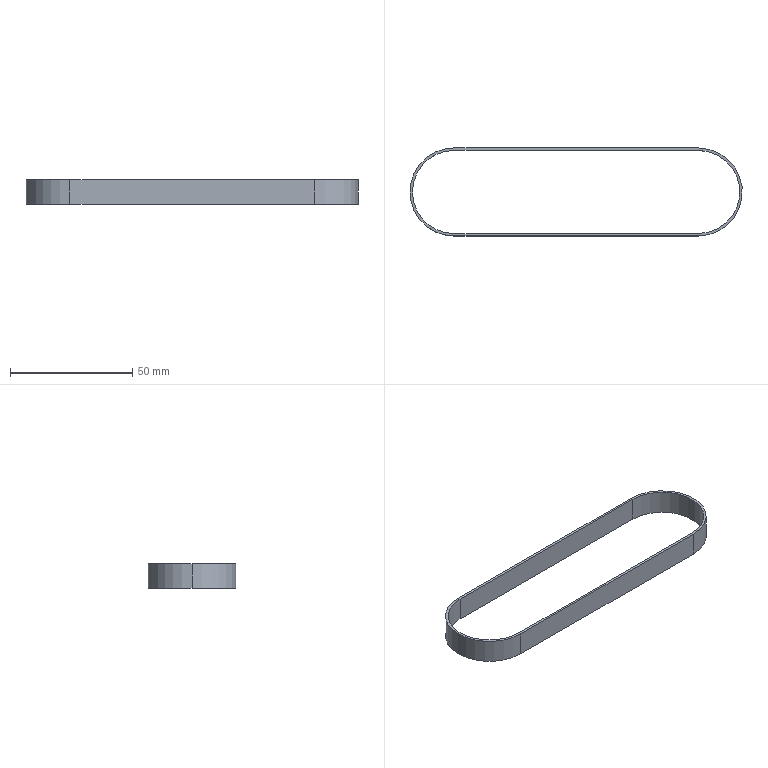Part | STEP file | Belt V1.201001 | 1 solid | 12 faces | box 136 x 36 x 10 mm | volume 3100 mm3 | cylinder 6 | plane 6 | commonest cylinder face diameters 34 x3 36 x3
STEP:
#1=CARTESIAN_POINT('',(0.,0.,0.));
#2=DIRECTION('',(0.,0.,1.));
#3=DIRECTION('',(1.,0.,0.));
#4=AXIS2_PLACEMENT_3D('',#1,#2,#3);
#5=CARTESIAN_POINT('',(-50.,17.,5.));
#6=VERTEX_POINT('',#5);
#7=CARTESIAN_POINT('',(-50.,17.,-5.));
#8=VERTEX_POINT('',#7);
#9=CARTESIAN_POINT('',(-50.,17.,5.));
#10=DIRECTION('',(0.,0.,-1.));
#11=VECTOR('',#10,1.);
#12=LINE('',#9,#11);
#13=CARTESIAN_POINT('',(-50.,0.,5.));
#14=DIRECTION('',(0.,0.,-1.));
#15=DIRECTION('',(-1.,0.,0.));
#16=AXIS2_PLACEMENT_3D('',#13,#14,#15);
#17=CYLINDRICAL_SURFACE('',#16,17.);
#18=CARTESIAN_POINT('',(1.571,0.));
#19=DIRECTION('',(0.,1.));
#20=VECTOR('',#19,1.);
#21=LINE('',#18,#20);
#22=(GEOMETRIC_REPRESENTATION_CONTEXT(2)PARAMETRIC_REPRESENTATION_CONTEXT()REPRESENTATION_CONTEXT('',''));
#23=DEFINITIONAL_REPRESENTATION('',(#21),#22);
#24=PCURVE('',#17,#23);
#25=CARTESIAN_POINT('',(-50.,17.,5.));
#26=DIRECTION('',(0.,-1.,0.));
#27=DIRECTION('',(0.,0.,-1.));
#28=AXIS2_PLACEMENT_3D('',#25,#26,#27);
#29=PLANE('',#28);
#30=CARTESIAN_POINT('',(0.,0.));
#31=DIRECTION('',(1.,0.));
#32=VECTOR('',#31,1.);
#33=LINE('',#30,#32);
#34=(GEOMETRIC_REPRESENTATION_CONTEXT(2)PARAMETRIC_REPRESENTATION_CONTEXT()REPRESENTATION_CONTEXT('',''));
#35=DEFINITIONAL_REPRESENTATION('',(#33),#34);
#36=PCURVE('',#29,#35);
#37=SURFACE_CURVE('',#12,(#24,#36),.PCURVE_S1.);
#38=EDGE_CURVE('',#6,#8,#37,.T.);
#39=ORIENTED_EDGE('',*,*,#38,.T.);
#40=CARTESIAN_POINT('',(-67.,0.,-5.));
#41=VERTEX_POINT('',#40);
#42=CARTESIAN_POINT('',(-50.,0.,-5.));
#43=DIRECTION('',(0.,0.,1.));
#44=DIRECTION('',(1.,0.,0.));
#45=AXIS2_PLACEMENT_3D('',#42,#43,#44);
#46=CIRCLE('',#45,17.);
#47=CARTESIAN_POINT('',(3.142,10.));
#48=DIRECTION('',(-1.,0.));
#49=VECTOR('',#48,1.);
#50=LINE('',#47,#49);
#51=(GEOMETRIC_REPRESENTATION_CONTEXT(2)PARAMETRIC_REPRESENTATION_CONTEXT()REPRESENTATION_CONTEXT('',''));
#52=DEFINITIONAL_REPRESENTATION('',(#50),#51);
#53=PCURVE('',#17,#52);
#54=CARTESIAN_POINT('',(-50.,0.,-5.));
#55=DIRECTION('',(0.,0.,1.));
#56=DIRECTION('',(1.,0.,0.));
#57=AXIS2_PLACEMENT_3D('',#54,#55,#56);
#58=PLANE('',#57);
#59=CARTESIAN_POINT('',(0.,0.));
#60=DIRECTION('',(1.,0.));
#61=AXIS2_PLACEMENT_2D('',#59,#60);
#62=CIRCLE('',#61,17.);
#63=(GEOMETRIC_REPRESENTATION_CONTEXT(2)PARAMETRIC_REPRESENTATION_CONTEXT()REPRESENTATION_CONTEXT('',''));
#64=DEFINITIONAL_REPRESENTATION('',(#62),#63);
#65=PCURVE('',#58,#64);
#66=SURFACE_CURVE('',#46,(#53,#65),.PCURVE_S1.);
#67=EDGE_CURVE('',#8,#41,#66,.T.);
#68=ORIENTED_EDGE('',*,*,#67,.T.);
#69=CARTESIAN_POINT('',(-67.,0.,5.));
#70=VERTEX_POINT('',#69);
#71=CARTESIAN_POINT('',(-67.,0.,5.));
#72=DIRECTION('',(0.,0.,-1.));
#73=VECTOR('',#72,1.);
#74=LINE('',#71,#73);
#75=CARTESIAN_POINT('',(0.,0.));
#76=DIRECTION('',(0.,1.));
#77=VECTOR('',#76,1.);
#78=LINE('',#75,#77);
#79=(GEOMETRIC_REPRESENTATION_CONTEXT(2)PARAMETRIC_REPRESENTATION_CONTEXT()REPRESENTATION_CONTEXT('',''));
#80=DEFINITIONAL_REPRESENTATION('',(#78),#79);
#81=PCURVE('',#17,#80);
#82=CARTESIAN_POINT('',(-50.,0.,5.));
#83=DIRECTION('',(0.,0.,-1.));
#84=DIRECTION('',(-1.,0.,0.));
#85=AXIS2_PLACEMENT_3D('',#82,#83,#84);
#86=CYLINDRICAL_SURFACE('',#85,17.);
#87=CARTESIAN_POINT('',(6.283,0.));
#88=DIRECTION('',(0.,1.));
#89=VECTOR('',#88,1.);
#90=LINE('',#87,#89);
#91=(GEOMETRIC_REPRESENTATION_CONTEXT(2)PARAMETRIC_REPRESENTATION_CONTEXT()REPRESENTATION_CONTEXT('',''));
#92=DEFINITIONAL_REPRESENTATION('',(#90),#91);
#93=PCURVE('',#86,#92);
#94=SURFACE_CURVE('',#74,(#81,#93),.PCURVE_S1.);
#95=EDGE_CURVE('',#70,#41,#94,.T.);
#96=ORIENTED_EDGE('',*,*,#95,.F.);
#97=CARTESIAN_POINT('',(-50.,0.,5.));
#98=DIRECTION('',(0.,0.,1.));
#99=DIRECTION('',(1.,0.,0.));
#100=AXIS2_PLACEMENT_3D('',#97,#98,#99);
#101=CIRCLE('',#100,17.);
#102=CARTESIAN_POINT('',(3.142,0.));
#103=DIRECTION('',(-1.,0.));
#104=VECTOR('',#103,1.);
#105=LINE('',#102,#104);
#106=(GEOMETRIC_REPRESENTATION_CONTEXT(2)PARAMETRIC_REPRESENTATION_CONTEXT()REPRESENTATION_CONTEXT('',''));
#107=DEFINITIONAL_REPRESENTATION('',(#105),#106);
#108=PCURVE('',#17,#107);
#109=CARTESIAN_POINT('',(-50.,0.,5.));
#110=DIRECTION('',(0.,0.,1.));
#111=DIRECTION('',(1.,0.,0.));
#112=AXIS2_PLACEMENT_3D('',#109,#110,#111);
#113=PLANE('',#112);
#114=CARTESIAN_POINT('',(0.,0.));
#115=DIRECTION('',(1.,0.));
#116=AXIS2_PLACEMENT_2D('',#114,#115);
#117=CIRCLE('',#116,17.);
#118=(GEOMETRIC_REPRESENTATION_CONTEXT(2)PARAMETRIC_REPRESENTATION_CONTEXT()REPRESENTATION_CONTEXT('',''));
#119=DEFINITIONAL_REPRESENTATION('',(#117),#118);
#120=PCURVE('',#113,#119);
#121=SURFACE_CURVE('',#101,(#108,#120),.PCURVE_S1.);
#122=EDGE_CURVE('',#6,#70,#121,.T.);
#123=ORIENTED_EDGE('',*,*,#122,.F.);
#124=EDGE_LOOP('',(#39,#68,#96,#123));
#125=FACE_BOUND('',#124,.F.);
#126=ADVANCED_FACE('',(#125),#17,.F.);
#127=CARTESIAN_POINT('',(-68.,0.,5.));
#128=VERTEX_POINT('',#127);
#129=CARTESIAN_POINT('',(-50.,-18.,5.));
#130=VERTEX_POINT('',#129);
#131=CARTESIAN_POINT('',(-50.,0.,5.));
#132=DIRECTION('',(0.,0.,1.));
#133=DIRECTION('',(1.,0.,0.));
#134=AXIS2_PLACEMENT_3D('',#131,#132,#133);
#135=CIRCLE('',#134,18.);
#136=CARTESIAN_POINT('',(-50.,0.,5.));
#137=DIRECTION('',(0.,0.,-1.));
#138=DIRECTION('',(-1.,0.,0.));
#139=AXIS2_PLACEMENT_3D('',#136,#137,#138);
#140=CYLINDRICAL_SURFACE('',#139,18.);
#141=CARTESIAN_POINT('',(9.425,0.));
#142=DIRECTION('',(-1.,0.));
#143=VECTOR('',#142,1.);
#144=LINE('',#141,#143);
#145=(GEOMETRIC_REPRESENTATION_CONTEXT(2)PARAMETRIC_REPRESENTATION_CONTEXT()REPRESENTATION_CONTEXT('',''));
#146=DEFINITIONAL_REPRESENTATION('',(#144),#145);
#147=PCURVE('',#140,#146);
#148=CARTESIAN_POINT('',(0.,0.));
#149=DIRECTION('',(1.,0.));
#150=AXIS2_PLACEMENT_2D('',#148,#149);
#151=CIRCLE('',#150,18.);
#152=(GEOMETRIC_REPRESENTATION_CONTEXT(2)PARAMETRIC_REPRESENTATION_CONTEXT()REPRESENTATION_CONTEXT('',''));
#153=DEFINITIONAL_REPRESENTATION('',(#151),#152);
#154=PCURVE('',#113,#153);
#155=SURFACE_CURVE('',#135,(#147,#154),.PCURVE_S1.);
#156=EDGE_CURVE('',#128,#130,#155,.T.);
#157=ORIENTED_EDGE('',*,*,#156,.F.);
#158=CARTESIAN_POINT('',(-68.,0.,-5.));
#159=VERTEX_POINT('',#158);
#160=CARTESIAN_POINT('',(-68.,0.,5.));
#161=DIRECTION('',(0.,0.,-1.));
#162=VECTOR('',#161,1.);
#163=LINE('',#160,#162);
#164=CARTESIAN_POINT('',(6.283,0.));
#165=DIRECTION('',(0.,1.));
#166=VECTOR('',#165,1.);
#167=LINE('',#164,#166);
#168=(GEOMETRIC_REPRESENTATION_CONTEXT(2)PARAMETRIC_REPRESENTATION_CONTEXT()REPRESENTATION_CONTEXT('',''));
#169=DEFINITIONAL_REPRESENTATION('',(#167),#168);
#170=PCURVE('',#140,#169);
#171=CARTESIAN_POINT('',(-50.,0.,5.));
#172=DIRECTION('',(0.,0.,-1.));
#173=DIRECTION('',(-1.,0.,0.));
#174=AXIS2_PLACEMENT_3D('',#171,#172,#173);
#175=CYLINDRICAL_SURFACE('',#174,18.);
#176=CARTESIAN_POINT('',(0.,0.));
#177=DIRECTION('',(0.,1.));
#178=VECTOR('',#177,1.);
#179=LINE('',#176,#178);
#180=(GEOMETRIC_REPRESENTATION_CONTEXT(2)PARAMETRIC_REPRESENTATION_CONTEXT()REPRESENTATION_CONTEXT('',''));
#181=DEFINITIONAL_REPRESENTATION('',(#179),#180);
#182=PCURVE('',#175,#181);
#183=SURFACE_CURVE('',#163,(#170,#182),.PCURVE_S1.);
#184=EDGE_CURVE('',#128,#159,#183,.T.);
#185=ORIENTED_EDGE('',*,*,#184,.T.);
#186=CARTESIAN_POINT('',(-50.,-18.,-5.));
#187=VERTEX_POINT('',#186);
#188=CARTESIAN_POINT('',(-50.,0.,-5.));
#189=DIRECTION('',(0.,0.,1.));
#190=DIRECTION('',(1.,0.,0.));
#191=AXIS2_PLACEMENT_3D('',#188,#189,#190);
#192=CIRCLE('',#191,18.);
#193=CARTESIAN_POINT('',(9.425,10.));
#194=DIRECTION('',(-1.,0.));
#195=VECTOR('',#194,1.);
#196=LINE('',#193,#195);
#197=(GEOMETRIC_REPRESENTATION_CONTEXT(2)PARAMETRIC_REPRESENTATION_CONTEXT()REPRESENTATION_CONTEXT('',''));
#198=DEFINITIONAL_REPRESENTATION('',(#196),#197);
#199=PCURVE('',#140,#198);
#200=CARTESIAN_POINT('',(0.,0.));
#201=DIRECTION('',(1.,0.));
#202=AXIS2_PLACEMENT_2D('',#200,#201);
#203=CIRCLE('',#202,18.);
#204=(GEOMETRIC_REPRESENTATION_CONTEXT(2)PARAMETRIC_REPRESENTATION_CONTEXT()REPRESENTATION_CONTEXT('',''));
#205=DEFINITIONAL_REPRESENTATION('',(#203),#204);
#206=PCURVE('',#58,#205);
#207=SURFACE_CURVE('',#192,(#199,#206),.PCURVE_S1.);
#208=EDGE_CURVE('',#159,#187,#207,.T.);
#209=ORIENTED_EDGE('',*,*,#208,.T.);
#210=CARTESIAN_POINT('',(-50.,-18.,5.));
#211=DIRECTION('',(0.,0.,-1.));
#212=VECTOR('',#211,1.);
#213=LINE('',#210,#212);
#214=CARTESIAN_POINT('',(4.712,0.));
#215=DIRECTION('',(0.,1.));
#216=VECTOR('',#215,1.);
#217=LINE('',#214,#216);
#218=(GEOMETRIC_REPRESENTATION_CONTEXT(2)PARAMETRIC_REPRESENTATION_CONTEXT()REPRESENTATION_CONTEXT('',''));
#219=DEFINITIONAL_REPRESENTATION('',(#217),#218);
#220=PCURVE('',#140,#219);
#221=CARTESIAN_POINT('',(-50.,-18.,5.));
#222=DIRECTION('',(0.,1.,0.));
#223=DIRECTION('',(0.,0.,1.));
#224=AXIS2_PLACEMENT_3D('',#221,#222,#223);
#225=PLANE('',#224);
#226=CARTESIAN_POINT('',(0.,0.));
#227=DIRECTION('',(-1.,0.));
#228=VECTOR('',#227,1.);
#229=LINE('',#226,#228);
#230=(GEOMETRIC_REPRESENTATION_CONTEXT(2)PARAMETRIC_REPRESENTATION_CONTEXT()REPRESENTATION_CONTEXT('',''));
#231=DEFINITIONAL_REPRESENTATION('',(#229),#230);
#232=PCURVE('',#225,#231);
#233=SURFACE_CURVE('',#213,(#220,#232),.PCURVE_S1.);
#234=EDGE_CURVE('',#130,#187,#233,.T.);
#235=ORIENTED_EDGE('',*,*,#234,.F.);
#236=EDGE_LOOP('',(#157,#185,#209,#235));
#237=FACE_BOUND('',#236,.T.);
#238=ADVANCED_FACE('',(#237),#140,.T.);
#239=CARTESIAN_POINT('',(-50.,18.,5.));
#240=VERTEX_POINT('',#239);
#241=CARTESIAN_POINT('',(-50.,0.,5.));
#242=DIRECTION('',(0.,0.,1.));
#243=DIRECTION('',(1.,0.,0.));
#244=AXIS2_PLACEMENT_3D('',#241,#242,#243);
#245=CIRCLE('',#244,18.);
#246=CARTESIAN_POINT('',(0.,0.));
#247=DIRECTION('',(1.,0.));
#248=AXIS2_PLACEMENT_2D('',#246,#247);
#249=CIRCLE('',#248,18.);
#250=(GEOMETRIC_REPRESENTATION_CONTEXT(2)PARAMETRIC_REPRESENTATION_CONTEXT()REPRESENTATION_CONTEXT('',''));
#251=DEFINITIONAL_REPRESENTATION('',(#249),#250);
#252=PCURVE('',#113,#251);
#253=CARTESIAN_POINT('',(3.142,0.));
#254=DIRECTION('',(-1.,0.));
#255=VECTOR('',#254,1.);
#256=LINE('',#253,#255);
#257=(GEOMETRIC_REPRESENTATION_CONTEXT(2)PARAMETRIC_REPRESENTATION_CONTEXT()REPRESENTATION_CONTEXT('',''));
#258=DEFINITIONAL_REPRESENTATION('',(#256),#257);
#259=PCURVE('',#175,#258);
#260=SURFACE_CURVE('',#245,(#252,#259),.PCURVE_S1.);
#261=EDGE_CURVE('',#240,#128,#260,.T.);
#262=ORIENTED_EDGE('',*,*,#261,.T.);
#263=ORIENTED_EDGE('',*,*,#156,.T.);
#264=CARTESIAN_POINT('',(50.,-18.,5.));
#265=VERTEX_POINT('',#264);
#266=CARTESIAN_POINT('',(-50.,-18.,5.));
#267=DIRECTION('',(1.,0.,0.));
#268=VECTOR('',#267,1.);
#269=LINE('',#266,#268);
#270=CARTESIAN_POINT('',(0.,-18.));
#271=DIRECTION('',(1.,0.));
#272=VECTOR('',#271,1.);
#273=LINE('',#270,#272);
#274=(GEOMETRIC_REPRESENTATION_CONTEXT(2)PARAMETRIC_REPRESENTATION_CONTEXT()REPRESENTATION_CONTEXT('',''));
#275=DEFINITIONAL_REPRESENTATION('',(#273),#274);
#276=PCURVE('',#113,#275);
#277=CARTESIAN_POINT('',(0.,0.));
#278=DIRECTION('',(0.,1.));
#279=VECTOR('',#278,1.);
#280=LINE('',#277,#279);
#281=(GEOMETRIC_REPRESENTATION_CONTEXT(2)PARAMETRIC_REPRESENTATION_CONTEXT()REPRESENTATION_CONTEXT('',''));
#282=DEFINITIONAL_REPRESENTATION('',(#280),#281);
#283=PCURVE('',#225,#282);
#284=SURFACE_CURVE('',#269,(#276,#283),.PCURVE_S1.);
#285=EDGE_CURVE('',#130,#265,#284,.T.);
#286=ORIENTED_EDGE('',*,*,#285,.T.);
#287=CARTESIAN_POINT('',(50.,18.,5.));
#288=VERTEX_POINT('',#287);
#289=CARTESIAN_POINT('',(50.,0.,5.));
#290=DIRECTION('',(0.,0.,1.));
#291=DIRECTION('',(1.,0.,0.));
#292=AXIS2_PLACEMENT_3D('',#289,#290,#291);
#293=CIRCLE('',#292,18.);
#294=CARTESIAN_POINT('',(100.,0.));
#295=DIRECTION('',(1.,0.));
#296=AXIS2_PLACEMENT_2D('',#294,#295);
#297=CIRCLE('',#296,18.);
#298=(GEOMETRIC_REPRESENTATION_CONTEXT(2)PARAMETRIC_REPRESENTATION_CONTEXT()REPRESENTATION_CONTEXT('',''));
#299=DEFINITIONAL_REPRESENTATION('',(#297),#298);
#300=PCURVE('',#113,#299);
#301=CARTESIAN_POINT('',(50.,0.,5.));
#302=DIRECTION('',(0.,0.,-1.));
#303=DIRECTION('',(-1.,0.,0.));
#304=AXIS2_PLACEMENT_3D('',#301,#302,#303);
#305=CYLINDRICAL_SURFACE('',#304,18.);
#306=CARTESIAN_POINT('',(9.425,0.));
#307=DIRECTION('',(-1.,0.));
#308=VECTOR('',#307,1.);
#309=LINE('',#306,#308);
#310=(GEOMETRIC_REPRESENTATION_CONTEXT(2)PARAMETRIC_REPRESENTATION_CONTEXT()REPRESENTATION_CONTEXT('',''));
#311=DEFINITIONAL_REPRESENTATION('',(#309),#310);
#312=PCURVE('',#305,#311);
#313=SURFACE_CURVE('',#293,(#300,#312),.PCURVE_S1.);
#314=EDGE_CURVE('',#265,#288,#313,.T.);
#315=ORIENTED_EDGE('',*,*,#314,.T.);
#316=CARTESIAN_POINT('',(-50.,18.,5.));
#317=DIRECTION('',(-1.,0.,0.));
#318=VECTOR('',#317,1.);
#319=LINE('',#316,#318);
#320=CARTESIAN_POINT('',(0.,18.));
#321=DIRECTION('',(-1.,0.));
#322=VECTOR('',#321,1.);
#323=LINE('',#320,#322);
#324=(GEOMETRIC_REPRESENTATION_CONTEXT(2)PARAMETRIC_REPRESENTATION_CONTEXT()REPRESENTATION_CONTEXT('',''));
#325=DEFINITIONAL_REPRESENTATION('',(#323),#324);
#326=PCURVE('',#113,#325);
#327=CARTESIAN_POINT('',(-50.,18.,5.));
#328=DIRECTION('',(0.,-1.,0.));
#329=DIRECTION('',(0.,0.,-1.));
#330=AXIS2_PLACEMENT_3D('',#327,#328,#329);
#331=PLANE('',#330);
#332=CARTESIAN_POINT('',(0.,0.));
#333=DIRECTION('',(0.,-1.));
#334=VECTOR('',#333,1.);
#335=LINE('',#332,#334);
#336=(GEOMETRIC_REPRESENTATION_CONTEXT(2)PARAMETRIC_REPRESENTATION_CONTEXT()REPRESENTATION_CONTEXT('',''));
#337=DEFINITIONAL_REPRESENTATION('',(#335),#336);
#338=PCURVE('',#331,#337);
#339=SURFACE_CURVE('',#319,(#326,#338),.PCURVE_S1.);
#340=EDGE_CURVE('',#288,#240,#339,.T.);
#341=ORIENTED_EDGE('',*,*,#340,.T.);
#342=EDGE_LOOP('',(#262,#263,#286,#315,#341));
#343=FACE_BOUND('',#342,.T.);
#344=CARTESIAN_POINT('',(-50.,-17.,5.));
#345=VERTEX_POINT('',#344);
#346=CARTESIAN_POINT('',(50.,-17.,5.));
#347=VERTEX_POINT('',#346);
#348=CARTESIAN_POINT('',(-50.,-17.,5.));
#349=DIRECTION('',(1.,0.,0.));
#350=VECTOR('',#349,1.);
#351=LINE('',#348,#350);
#352=CARTESIAN_POINT('',(0.,-17.));
#353=DIRECTION('',(1.,0.));
#354=VECTOR('',#353,1.);
#355=LINE('',#352,#354);
#356=(GEOMETRIC_REPRESENTATION_CONTEXT(2)PARAMETRIC_REPRESENTATION_CONTEXT()REPRESENTATION_CONTEXT('',''));
#357=DEFINITIONAL_REPRESENTATION('',(#355),#356);
#358=PCURVE('',#113,#357);
#359=CARTESIAN_POINT('',(-50.,-17.,5.));
#360=DIRECTION('',(0.,1.,0.));
#361=DIRECTION('',(0.,0.,1.));
#362=AXIS2_PLACEMENT_3D('',#359,#360,#361);
#363=PLANE('',#362);
#364=CARTESIAN_POINT('',(0.,0.));
#365=DIRECTION('',(0.,1.));
#366=VECTOR('',#365,1.);
#367=LINE('',#364,#366);
#368=(GEOMETRIC_REPRESENTATION_CONTEXT(2)PARAMETRIC_REPRESENTATION_CONTEXT()REPRESENTATION_CONTEXT('',''));
#369=DEFINITIONAL_REPRESENTATION('',(#367),#368);
#370=PCURVE('',#363,#369);
#371=SURFACE_CURVE('',#351,(#358,#370),.PCURVE_S1.);
#372=EDGE_CURVE('',#345,#347,#371,.T.);
#373=ORIENTED_EDGE('',*,*,#372,.F.);
#374=CARTESIAN_POINT('',(-50.,0.,5.));
#375=DIRECTION('',(0.,0.,1.));
#376=DIRECTION('',(1.,0.,0.));
#377=AXIS2_PLACEMENT_3D('',#374,#375,#376);
#378=CIRCLE('',#377,17.);
#379=CARTESIAN_POINT('',(0.,0.));
#380=DIRECTION('',(1.,0.));
#381=AXIS2_PLACEMENT_2D('',#379,#380);
#382=CIRCLE('',#381,17.);
#383=(GEOMETRIC_REPRESENTATION_CONTEXT(2)PARAMETRIC_REPRESENTATION_CONTEXT()REPRESENTATION_CONTEXT('',''));
#384=DEFINITIONAL_REPRESENTATION('',(#382),#383);
#385=PCURVE('',#113,#384);
#386=CARTESIAN_POINT('',(9.425,0.));
#387=DIRECTION('',(-1.,0.));
#388=VECTOR('',#387,1.);
#389=LINE('',#386,#388);
#390=(GEOMETRIC_REPRESENTATION_CONTEXT(2)PARAMETRIC_REPRESENTATION_CONTEXT()REPRESENTATION_CONTEXT('',''));
#391=DEFINITIONAL_REPRESENTATION('',(#389),#390);
#392=PCURVE('',#86,#391);
#393=SURFACE_CURVE('',#378,(#385,#392),.PCURVE_S1.);
#394=EDGE_CURVE('',#70,#345,#393,.T.);
#395=ORIENTED_EDGE('',*,*,#394,.F.);
#396=ORIENTED_EDGE('',*,*,#122,.F.);
#397=CARTESIAN_POINT('',(50.,17.,5.));
#398=VERTEX_POINT('',#397);
#399=CARTESIAN_POINT('',(-50.,17.,5.));
#400=DIRECTION('',(-1.,0.,0.));
#401=VECTOR('',#400,1.);
#402=LINE('',#399,#401);
#403=CARTESIAN_POINT('',(0.,17.));
#404=DIRECTION('',(-1.,0.));
#405=VECTOR('',#404,1.);
#406=LINE('',#403,#405);
#407=(GEOMETRIC_REPRESENTATION_CONTEXT(2)PARAMETRIC_REPRESENTATION_CONTEXT()REPRESENTATION_CONTEXT('',''));
#408=DEFINITIONAL_REPRESENTATION('',(#406),#407);
#409=PCURVE('',#113,#408);
#410=CARTESIAN_POINT('',(0.,0.));
#411=DIRECTION('',(0.,-1.));
#412=VECTOR('',#411,1.);
#413=LINE('',#410,#412);
#414=(GEOMETRIC_REPRESENTATION_CONTEXT(2)PARAMETRIC_REPRESENTATION_CONTEXT()REPRESENTATION_CONTEXT('',''));
#415=DEFINITIONAL_REPRESENTATION('',(#413),#414);
#416=PCURVE('',#29,#415);
#417=SURFACE_CURVE('',#402,(#409,#416),.PCURVE_S1.);
#418=EDGE_CURVE('',#398,#6,#417,.T.);
#419=ORIENTED_EDGE('',*,*,#418,.F.);
#420=CARTESIAN_POINT('',(50.,0.,5.));
#421=DIRECTION('',(0.,0.,1.));
#422=DIRECTION('',(-1.,0.,0.));
#423=AXIS2_PLACEMENT_3D('',#420,#421,#422);
#424=CIRCLE('',#423,17.);
#425=CARTESIAN_POINT('',(100.,0.));
#426=DIRECTION('',(-1.,0.));
#427=AXIS2_PLACEMENT_2D('',#425,#426);
#428=CIRCLE('',#427,17.);
#429=(GEOMETRIC_REPRESENTATION_CONTEXT(2)PARAMETRIC_REPRESENTATION_CONTEXT()REPRESENTATION_CONTEXT('',''));
#430=DEFINITIONAL_REPRESENTATION('',(#428),#429);
#431=PCURVE('',#113,#430);
#432=CARTESIAN_POINT('',(50.,0.,5.));
#433=DIRECTION('',(0.,0.,-1.));
#434=DIRECTION('',(-1.,0.,0.));
#435=AXIS2_PLACEMENT_3D('',#432,#433,#434);
#436=CYLINDRICAL_SURFACE('',#435,17.);
#437=CARTESIAN_POINT('',(6.283,0.));
#438=DIRECTION('',(-1.,0.));
#439=VECTOR('',#438,1.);
#440=LINE('',#437,#439);
#441=(GEOMETRIC_REPRESENTATION_CONTEXT(2)PARAMETRIC_REPRESENTATION_CONTEXT()REPRESENTATION_CONTEXT('',''));
#442=DEFINITIONAL_REPRESENTATION('',(#440),#441);
#443=PCURVE('',#436,#442);
#444=SURFACE_CURVE('',#424,(#431,#443),.PCURVE_S1.);
#445=EDGE_CURVE('',#347,#398,#444,.T.);
#446=ORIENTED_EDGE('',*,*,#445,.F.);
#447=EDGE_LOOP('',(#373,#395,#396,#419,#446));
#448=FACE_BOUND('',#447,.T.);
#449=ADVANCED_FACE('',(#343,#448),#113,.T.);
#450=CARTESIAN_POINT('',(-50.,18.,-5.));
#451=VERTEX_POINT('',#450);
#452=CARTESIAN_POINT('',(-50.,0.,-5.));
#453=DIRECTION('',(0.,0.,1.));
#454=DIRECTION('',(1.,0.,0.));
#455=AXIS2_PLACEMENT_3D('',#452,#453,#454);
#456=CIRCLE('',#455,18.);
#457=CARTESIAN_POINT('',(0.,0.));
#458=DIRECTION('',(1.,0.));
#459=AXIS2_PLACEMENT_2D('',#457,#458);
#460=CIRCLE('',#459,18.);
#461=(GEOMETRIC_REPRESENTATION_CONTEXT(2)PARAMETRIC_REPRESENTATION_CONTEXT()REPRESENTATION_CONTEXT('',''));
#462=DEFINITIONAL_REPRESENTATION('',(#460),#461);
#463=PCURVE('',#58,#462);
#464=CARTESIAN_POINT('',(3.142,10.));
#465=DIRECTION('',(-1.,0.));
#466=VECTOR('',#465,1.);
#467=LINE('',#464,#466);
#468=(GEOMETRIC_REPRESENTATION_CONTEXT(2)PARAMETRIC_REPRESENTATION_CONTEXT()REPRESENTATION_CONTEXT('',''));
#469=DEFINITIONAL_REPRESENTATION('',(#467),#468);
#470=PCURVE('',#175,#469);
#471=SURFACE_CURVE('',#456,(#463,#470),.PCURVE_S1.);
#472=EDGE_CURVE('',#451,#159,#471,.T.);
#473=ORIENTED_EDGE('',*,*,#472,.F.);
#474=CARTESIAN_POINT('',(50.,18.,-5.));
#475=VERTEX_POINT('',#474);
#476=CARTESIAN_POINT('',(-50.,18.,-5.));
#477=DIRECTION('',(-1.,0.,0.));
#478=VECTOR('',#477,1.);
#479=LINE('',#476,#478);
#480=CARTESIAN_POINT('',(0.,18.));
#481=DIRECTION('',(-1.,0.));
#482=VECTOR('',#481,1.);
#483=LINE('',#480,#482);
#484=(GEOMETRIC_REPRESENTATION_CONTEXT(2)PARAMETRIC_REPRESENTATION_CONTEXT()REPRESENTATION_CONTEXT('',''));
#485=DEFINITIONAL_REPRESENTATION('',(#483),#484);
#486=PCURVE('',#58,#485);
#487=CARTESIAN_POINT('',(10.,0.));
#488=DIRECTION('',(0.,-1.));
#489=VECTOR('',#488,1.);
#490=LINE('',#487,#489);
#491=(GEOMETRIC_REPRESENTATION_CONTEXT(2)PARAMETRIC_REPRESENTATION_CONTEXT()REPRESENTATION_CONTEXT('',''));
#492=DEFINITIONAL_REPRESENTATION('',(#490),#491);
#493=PCURVE('',#331,#492);
#494=SURFACE_CURVE('',#479,(#486,#493),.PCURVE_S1.);
#495=EDGE_CURVE('',#475,#451,#494,.T.);
#496=ORIENTED_EDGE('',*,*,#495,.F.);
#497=CARTESIAN_POINT('',(50.,-18.,-5.));
#498=VERTEX_POINT('',#497);
#499=CARTESIAN_POINT('',(50.,0.,-5.));
#500=DIRECTION('',(0.,0.,1.));
#501=DIRECTION('',(1.,0.,0.));
#502=AXIS2_PLACEMENT_3D('',#499,#500,#501);
#503=CIRCLE('',#502,18.);
#504=CARTESIAN_POINT('',(100.,0.));
#505=DIRECTION('',(1.,0.));
#506=AXIS2_PLACEMENT_2D('',#504,#505);
#507=CIRCLE('',#506,18.);
#508=(GEOMETRIC_REPRESENTATION_CONTEXT(2)PARAMETRIC_REPRESENTATION_CONTEXT()REPRESENTATION_CONTEXT('',''));
#509=DEFINITIONAL_REPRESENTATION('',(#507),#508);
#510=PCURVE('',#58,#509);
#511=CARTESIAN_POINT('',(9.425,10.));
#512=DIRECTION('',(-1.,0.));
#513=VECTOR('',#512,1.);
#514=LINE('',#511,#513);
#515=(GEOMETRIC_REPRESENTATION_CONTEXT(2)PARAMETRIC_REPRESENTATION_CONTEXT()REPRESENTATION_CONTEXT('',''));
#516=DEFINITIONAL_REPRESENTATION('',(#514),#515);
#517=PCURVE('',#305,#516);
#518=SURFACE_CURVE('',#503,(#510,#517),.PCURVE_S1.);
#519=EDGE_CURVE('',#498,#475,#518,.T.);
#520=ORIENTED_EDGE('',*,*,#519,.F.);
#521=CARTESIAN_POINT('',(-50.,-18.,-5.));
#522=DIRECTION('',(1.,0.,0.));
#523=VECTOR('',#522,1.);
#524=LINE('',#521,#523);
#525=CARTESIAN_POINT('',(0.,-18.));
#526=DIRECTION('',(1.,0.));
#527=VECTOR('',#526,1.);
#528=LINE('',#525,#527);
#529=(GEOMETRIC_REPRESENTATION_CONTEXT(2)PARAMETRIC_REPRESENTATION_CONTEXT()REPRESENTATION_CONTEXT('',''));
#530=DEFINITIONAL_REPRESENTATION('',(#528),#529);
#531=PCURVE('',#58,#530);
#532=CARTESIAN_POINT('',(-10.,0.));
#533=DIRECTION('',(0.,1.));
#534=VECTOR('',#533,1.);
#535=LINE('',#532,#534);
#536=(GEOMETRIC_REPRESENTATION_CONTEXT(2)PARAMETRIC_REPRESENTATION_CONTEXT()REPRESENTATION_CONTEXT('',''));
#537=DEFINITIONAL_REPRESENTATION('',(#535),#536);
#538=PCURVE('',#225,#537);
#539=SURFACE_CURVE('',#524,(#531,#538),.PCURVE_S1.);
#540=EDGE_CURVE('',#187,#498,#539,.T.);
#541=ORIENTED_EDGE('',*,*,#540,.F.);
#542=ORIENTED_EDGE('',*,*,#208,.F.);
#543=EDGE_LOOP('',(#473,#496,#520,#541,#542));
#544=FACE_BOUND('',#543,.T.);
#545=ORIENTED_EDGE('',*,*,#67,.T.);
#546=CARTESIAN_POINT('',(-50.,-17.,-5.));
#547=VERTEX_POINT('',#546);
#548=CARTESIAN_POINT('',(-50.,0.,-5.));
#549=DIRECTION('',(0.,0.,1.));
#550=DIRECTION('',(1.,0.,0.));
#551=AXIS2_PLACEMENT_3D('',#548,#549,#550);
#552=CIRCLE('',#551,17.);
#553=CARTESIAN_POINT('',(0.,0.));
#554=DIRECTION('',(1.,0.));
#555=AXIS2_PLACEMENT_2D('',#553,#554);
#556=CIRCLE('',#555,17.);
#557=(GEOMETRIC_REPRESENTATION_CONTEXT(2)PARAMETRIC_REPRESENTATION_CONTEXT()REPRESENTATION_CONTEXT('',''));
#558=DEFINITIONAL_REPRESENTATION('',(#556),#557);
#559=PCURVE('',#58,#558);
#560=CARTESIAN_POINT('',(9.425,10.));
#561=DIRECTION('',(-1.,0.));
#562=VECTOR('',#561,1.);
#563=LINE('',#560,#562);
#564=(GEOMETRIC_REPRESENTATION_CONTEXT(2)PARAMETRIC_REPRESENTATION_CONTEXT()REPRESENTATION_CONTEXT('',''));
#565=DEFINITIONAL_REPRESENTATION('',(#563),#564);
#566=PCURVE('',#86,#565);
#567=SURFACE_CURVE('',#552,(#559,#566),.PCURVE_S1.);
#568=EDGE_CURVE('',#41,#547,#567,.T.);
#569=ORIENTED_EDGE('',*,*,#568,.T.);
#570=CARTESIAN_POINT('',(50.,-17.,-5.));
#571=VERTEX_POINT('',#570);
#572=CARTESIAN_POINT('',(-50.,-17.,-5.));
#573=DIRECTION('',(1.,0.,0.));
#574=VECTOR('',#573,1.);
#575=LINE('',#572,#574);
#576=CARTESIAN_POINT('',(0.,-17.));
#577=DIRECTION('',(1.,0.));
#578=VECTOR('',#577,1.);
#579=LINE('',#576,#578);
#580=(GEOMETRIC_REPRESENTATION_CONTEXT(2)PARAMETRIC_REPRESENTATION_CONTEXT()REPRESENTATION_CONTEXT('',''));
#581=DEFINITIONAL_REPRESENTATION('',(#579),#580);
#582=PCURVE('',#58,#581);
#583=CARTESIAN_POINT('',(-10.,0.));
#584=DIRECTION('',(0.,1.));
#585=VECTOR('',#584,1.);
#586=LINE('',#583,#585);
#587=(GEOMETRIC_REPRESENTATION_CONTEXT(2)PARAMETRIC_REPRESENTATION_CONTEXT()REPRESENTATION_CONTEXT('',''));
#588=DEFINITIONAL_REPRESENTATION('',(#586),#587);
#589=PCURVE('',#363,#588);
#590=SURFACE_CURVE('',#575,(#582,#589),.PCURVE_S1.);
#591=EDGE_CURVE('',#547,#571,#590,.T.);
#592=ORIENTED_EDGE('',*,*,#591,.T.);
#593=CARTESIAN_POINT('',(50.,17.,-5.));
#594=VERTEX_POINT('',#593);
#595=CARTESIAN_POINT('',(50.,0.,-5.));
#596=DIRECTION('',(0.,0.,1.));
#597=DIRECTION('',(-1.,0.,0.));
#598=AXIS2_PLACEMENT_3D('',#595,#596,#597);
#599=CIRCLE('',#598,17.);
#600=CARTESIAN_POINT('',(100.,0.));
#601=DIRECTION('',(-1.,0.));
#602=AXIS2_PLACEMENT_2D('',#600,#601);
#603=CIRCLE('',#602,17.);
#604=(GEOMETRIC_REPRESENTATION_CONTEXT(2)PARAMETRIC_REPRESENTATION_CONTEXT()REPRESENTATION_CONTEXT('',''));
#605=DEFINITIONAL_REPRESENTATION('',(#603),#604);
#606=PCURVE('',#58,#605);
#607=CARTESIAN_POINT('',(6.283,10.));
#608=DIRECTION('',(-1.,0.));
#609=VECTOR('',#608,1.);
#610=LINE('',#607,#609);
#611=(GEOMETRIC_REPRESENTATION_CONTEXT(2)PARAMETRIC_REPRESENTATION_CONTEXT()REPRESENTATION_CONTEXT('',''));
#612=DEFINITIONAL_REPRESENTATION('',(#610),#611);
#613=PCURVE('',#436,#612);
#614=SURFACE_CURVE('',#599,(#606,#613),.PCURVE_S1.);
#615=EDGE_CURVE('',#571,#594,#614,.T.);
#616=ORIENTED_EDGE('',*,*,#615,.T.);
#617=CARTESIAN_POINT('',(-50.,17.,-5.));
#618=DIRECTION('',(-1.,0.,0.));
#619=VECTOR('',#618,1.);
#620=LINE('',#617,#619);
#621=CARTESIAN_POINT('',(0.,17.));
#622=DIRECTION('',(-1.,0.));
#623=VECTOR('',#622,1.);
#624=LINE('',#621,#623);
#625=(GEOMETRIC_REPRESENTATION_CONTEXT(2)PARAMETRIC_REPRESENTATION_CONTEXT()REPRESENTATION_CONTEXT('',''));
#626=DEFINITIONAL_REPRESENTATION('',(#624),#625);
#627=PCURVE('',#58,#626);
#628=CARTESIAN_POINT('',(10.,0.));
#629=DIRECTION('',(0.,-1.));
#630=VECTOR('',#629,1.);
#631=LINE('',#628,#630);
#632=(GEOMETRIC_REPRESENTATION_CONTEXT(2)PARAMETRIC_REPRESENTATION_CONTEXT()REPRESENTATION_CONTEXT('',''));
#633=DEFINITIONAL_REPRESENTATION('',(#631),#632);
#634=PCURVE('',#29,#633);
#635=SURFACE_CURVE('',#620,(#627,#634),.PCURVE_S1.);
#636=EDGE_CURVE('',#594,#8,#635,.T.);
#637=ORIENTED_EDGE('',*,*,#636,.T.);
#638=EDGE_LOOP('',(#545,#569,#592,#616,#637));
#639=FACE_BOUND('',#638,.T.);
#640=ADVANCED_FACE('',(#544,#639),#58,.F.);
#641=ORIENTED_EDGE('',*,*,#184,.F.);
#642=ORIENTED_EDGE('',*,*,#261,.F.);
#643=CARTESIAN_POINT('',(-50.,18.,5.));
#644=DIRECTION('',(0.,0.,-1.));
#645=VECTOR('',#644,1.);
#646=LINE('',#643,#645);
#647=CARTESIAN_POINT('',(1.571,0.));
#648=DIRECTION('',(0.,1.));
#649=VECTOR('',#648,1.);
#650=LINE('',#647,#649);
#651=(GEOMETRIC_REPRESENTATION_CONTEXT(2)PARAMETRIC_REPRESENTATION_CONTEXT()REPRESENTATION_CONTEXT('',''));
#652=DEFINITIONAL_REPRESENTATION('',(#650),#651);
#653=PCURVE('',#175,#652);
#654=CARTESIAN_POINT('',(0.,0.));
#655=DIRECTION('',(1.,0.));
#656=VECTOR('',#655,1.);
#657=LINE('',#654,#656);
#658=(GEOMETRIC_REPRESENTATION_CONTEXT(2)PARAMETRIC_REPRESENTATION_CONTEXT()REPRESENTATION_CONTEXT('',''));
#659=DEFINITIONAL_REPRESENTATION('',(#657),#658);
#660=PCURVE('',#331,#659);
#661=SURFACE_CURVE('',#646,(#653,#660),.PCURVE_S1.);
#662=EDGE_CURVE('',#240,#451,#661,.T.);
#663=ORIENTED_EDGE('',*,*,#662,.T.);
#664=ORIENTED_EDGE('',*,*,#472,.T.);
#665=EDGE_LOOP('',(#641,#642,#663,#664));
#666=FACE_BOUND('',#665,.T.);
#667=ADVANCED_FACE('',(#666),#175,.T.);
#668=ORIENTED_EDGE('',*,*,#540,.T.);
#669=CARTESIAN_POINT('',(50.,-18.,5.));
#670=DIRECTION('',(0.,0.,-1.));
#671=VECTOR('',#670,1.);
#672=LINE('',#669,#671);
#673=CARTESIAN_POINT('',(0.,100.));
#674=DIRECTION('',(-1.,0.));
#675=VECTOR('',#674,1.);
#676=LINE('',#673,#675);
#677=(GEOMETRIC_REPRESENTATION_CONTEXT(2)PARAMETRIC_REPRESENTATION_CONTEXT()REPRESENTATION_CONTEXT('',''));
#678=DEFINITIONAL_REPRESENTATION('',(#676),#677);
#679=PCURVE('',#225,#678);
#680=CARTESIAN_POINT('',(4.712,0.));
#681=DIRECTION('',(0.,1.));
#682=VECTOR('',#681,1.);
#683=LINE('',#680,#682);
#684=(GEOMETRIC_REPRESENTATION_CONTEXT(2)PARAMETRIC_REPRESENTATION_CONTEXT()REPRESENTATION_CONTEXT('',''));
#685=DEFINITIONAL_REPRESENTATION('',(#683),#684);
#686=PCURVE('',#305,#685);
#687=SURFACE_CURVE('',#672,(#679,#686),.PCURVE_S1.);
#688=EDGE_CURVE('',#265,#498,#687,.T.);
#689=ORIENTED_EDGE('',*,*,#688,.F.);
#690=ORIENTED_EDGE('',*,*,#285,.F.);
#691=ORIENTED_EDGE('',*,*,#234,.T.);
#692=EDGE_LOOP('',(#668,#689,#690,#691));
#693=FACE_BOUND('',#692,.T.);
#694=ADVANCED_FACE('',(#693),#225,.F.);
#695=ORIENTED_EDGE('',*,*,#519,.T.);
#696=CARTESIAN_POINT('',(50.,18.,5.));
#697=DIRECTION('',(0.,0.,-1.));
#698=VECTOR('',#697,1.);
#699=LINE('',#696,#698);
#700=CARTESIAN_POINT('',(1.571,0.));
#701=DIRECTION('',(0.,1.));
#702=VECTOR('',#701,1.);
#703=LINE('',#700,#702);
#704=(GEOMETRIC_REPRESENTATION_CONTEXT(2)PARAMETRIC_REPRESENTATION_CONTEXT()REPRESENTATION_CONTEXT('',''));
#705=DEFINITIONAL_REPRESENTATION('',(#703),#704);
#706=PCURVE('',#305,#705);
#707=CARTESIAN_POINT('',(0.,100.));
#708=DIRECTION('',(1.,0.));
#709=VECTOR('',#708,1.);
#710=LINE('',#707,#709);
#711=(GEOMETRIC_REPRESENTATION_CONTEXT(2)PARAMETRIC_REPRESENTATION_CONTEXT()REPRESENTATION_CONTEXT('',''));
#712=DEFINITIONAL_REPRESENTATION('',(#710),#711);
#713=PCURVE('',#331,#712);
#714=SURFACE_CURVE('',#699,(#706,#713),.PCURVE_S1.);
#715=EDGE_CURVE('',#288,#475,#714,.T.);
#716=ORIENTED_EDGE('',*,*,#715,.F.);
#717=ORIENTED_EDGE('',*,*,#314,.F.);
#718=ORIENTED_EDGE('',*,*,#688,.T.);
#719=EDGE_LOOP('',(#695,#716,#717,#718));
#720=FACE_BOUND('',#719,.T.);
#721=ADVANCED_FACE('',(#720),#305,.T.);
#722=ORIENTED_EDGE('',*,*,#495,.T.);
#723=ORIENTED_EDGE('',*,*,#662,.F.);
#724=ORIENTED_EDGE('',*,*,#340,.F.);
#725=ORIENTED_EDGE('',*,*,#715,.T.);
#726=EDGE_LOOP('',(#722,#723,#724,#725));
#727=FACE_BOUND('',#726,.T.);
#728=ADVANCED_FACE('',(#727),#331,.F.);
#729=ORIENTED_EDGE('',*,*,#568,.T.);
#730=CARTESIAN_POINT('',(-50.,-17.,5.));
#731=DIRECTION('',(0.,0.,-1.));
#732=VECTOR('',#731,1.);
#733=LINE('',#730,#732);
#734=CARTESIAN_POINT('',(4.712,0.));
#735=DIRECTION('',(0.,1.));
#736=VECTOR('',#735,1.);
#737=LINE('',#734,#736);
#738=(GEOMETRIC_REPRESENTATION_CONTEXT(2)PARAMETRIC_REPRESENTATION_CONTEXT()REPRESENTATION_CONTEXT('',''));
#739=DEFINITIONAL_REPRESENTATION('',(#737),#738);
#740=PCURVE('',#86,#739);
#741=CARTESIAN_POINT('',(0.,0.));
#742=DIRECTION('',(-1.,0.));
#743=VECTOR('',#742,1.);
#744=LINE('',#741,#743);
#745=(GEOMETRIC_REPRESENTATION_CONTEXT(2)PARAMETRIC_REPRESENTATION_CONTEXT()REPRESENTATION_CONTEXT('',''));
#746=DEFINITIONAL_REPRESENTATION('',(#744),#745);
#747=PCURVE('',#363,#746);
#748=SURFACE_CURVE('',#733,(#740,#747),.PCURVE_S1.);
#749=EDGE_CURVE('',#345,#547,#748,.T.);
#750=ORIENTED_EDGE('',*,*,#749,.F.);
#751=ORIENTED_EDGE('',*,*,#394,.F.);
#752=ORIENTED_EDGE('',*,*,#95,.T.);
#753=EDGE_LOOP('',(#729,#750,#751,#752));
#754=FACE_BOUND('',#753,.F.);
#755=ADVANCED_FACE('',(#754),#86,.F.);
#756=ORIENTED_EDGE('',*,*,#591,.F.);
#757=ORIENTED_EDGE('',*,*,#749,.F.);
#758=ORIENTED_EDGE('',*,*,#372,.T.);
#759=CARTESIAN_POINT('',(50.,-17.,5.));
#760=DIRECTION('',(0.,0.,-1.));
#761=VECTOR('',#760,1.);
#762=LINE('',#759,#761);
#763=CARTESIAN_POINT('',(0.,100.));
#764=DIRECTION('',(-1.,0.));
#765=VECTOR('',#764,1.);
#766=LINE('',#763,#765);
#767=(GEOMETRIC_REPRESENTATION_CONTEXT(2)PARAMETRIC_REPRESENTATION_CONTEXT()REPRESENTATION_CONTEXT('',''));
#768=DEFINITIONAL_REPRESENTATION('',(#766),#767);
#769=PCURVE('',#363,#768);
#770=CARTESIAN_POINT('',(4.712,0.));
#771=DIRECTION('',(0.,1.));
#772=VECTOR('',#771,1.);
#773=LINE('',#770,#772);
#774=(GEOMETRIC_REPRESENTATION_CONTEXT(2)PARAMETRIC_REPRESENTATION_CONTEXT()REPRESENTATION_CONTEXT('',''));
#775=DEFINITIONAL_REPRESENTATION('',(#773),#774);
#776=PCURVE('',#436,#775);
#777=SURFACE_CURVE('',#762,(#769,#776),.PCURVE_S1.);
#778=EDGE_CURVE('',#347,#571,#777,.T.);
#779=ORIENTED_EDGE('',*,*,#778,.T.);
#780=EDGE_LOOP('',(#756,#757,#758,#779));
#781=FACE_BOUND('',#780,.T.);
#782=ADVANCED_FACE('',(#781),#363,.T.);
#783=CARTESIAN_POINT('',(50.,17.,5.));
#784=DIRECTION('',(0.,0.,-1.));
#785=VECTOR('',#784,1.);
#786=LINE('',#783,#785);
#787=CARTESIAN_POINT('',(1.571,0.));
#788=DIRECTION('',(0.,1.));
#789=VECTOR('',#788,1.);
#790=LINE('',#787,#789);
#791=(GEOMETRIC_REPRESENTATION_CONTEXT(2)PARAMETRIC_REPRESENTATION_CONTEXT()REPRESENTATION_CONTEXT('',''));
#792=DEFINITIONAL_REPRESENTATION('',(#790),#791);
#793=PCURVE('',#436,#792);
#794=CARTESIAN_POINT('',(0.,100.));
#795=DIRECTION('',(1.,0.));
#796=VECTOR('',#795,1.);
#797=LINE('',#794,#796);
#798=(GEOMETRIC_REPRESENTATION_CONTEXT(2)PARAMETRIC_REPRESENTATION_CONTEXT()REPRESENTATION_CONTEXT('',''));
#799=DEFINITIONAL_REPRESENTATION('',(#797),#798);
#800=PCURVE('',#29,#799);
#801=SURFACE_CURVE('',#786,(#793,#800),.PCURVE_S1.);
#802=EDGE_CURVE('',#398,#594,#801,.T.);
#803=ORIENTED_EDGE('',*,*,#802,.F.);
#804=ORIENTED_EDGE('',*,*,#445,.F.);
#805=ORIENTED_EDGE('',*,*,#778,.T.);
#806=ORIENTED_EDGE('',*,*,#615,.T.);
#807=EDGE_LOOP('',(#803,#804,#805,#806));
#808=FACE_BOUND('',#807,.F.);
#809=ADVANCED_FACE('',(#808),#436,.F.);
#810=ORIENTED_EDGE('',*,*,#636,.F.);
#811=ORIENTED_EDGE('',*,*,#802,.F.);
#812=ORIENTED_EDGE('',*,*,#418,.T.);
#813=ORIENTED_EDGE('',*,*,#38,.T.);
#814=EDGE_LOOP('',(#810,#811,#812,#813));
#815=FACE_BOUND('',#814,.T.);
#816=ADVANCED_FACE('',(#815),#29,.T.);
#817=CLOSED_SHELL('',(#126,#238,#449,#640,#667,#694,#721,#728,#755,#782,#809,#816));
#818=MANIFOLD_SOLID_BREP('',#817);
#819=(LENGTH_UNIT()NAMED_UNIT(*)SI_UNIT(.MILLI.,.METRE.));
#820=UNCERTAINTY_MEASURE_WITH_UNIT(LENGTH_MEASURE(0.0000001),#819,'','');
#821=(NAMED_UNIT(*)PLANE_ANGLE_UNIT()SI_UNIT($,.RADIAN.));
#822=(NAMED_UNIT(*)SI_UNIT($,.STERADIAN.)SOLID_ANGLE_UNIT());
#823=(GEOMETRIC_REPRESENTATION_CONTEXT(3)GLOBAL_UNCERTAINTY_ASSIGNED_CONTEXT((#820))GLOBAL_UNIT_ASSIGNED_CONTEXT((#819,#821,#822))REPRESENTATION_CONTEXT('',''));
#824=ADVANCED_BREP_SHAPE_REPRESENTATION('',(#4,#818),#823);